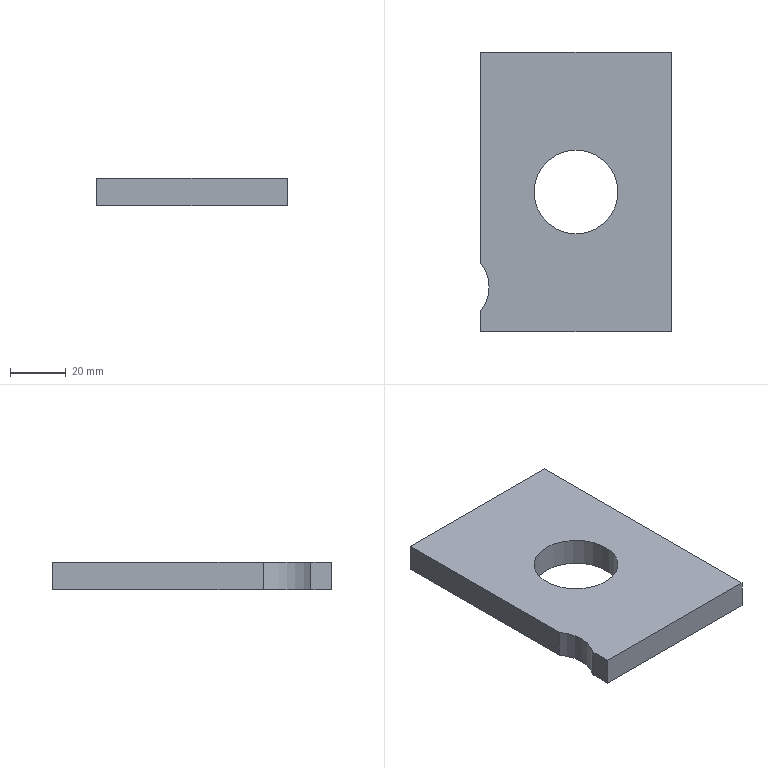Part | NX | features solid 2 | 1 solid | 9 faces | box 68 x 100 x 10 mm | volume 60595 mm3 | plane 7 | cylinder 2 | commonest cylinder face diameters 28 x1 30 x1
STEP:
#1=CARTESIAN_POINT('',(-550.,-16.475,-180.));
#2=VERTEX_POINT('',#1);
#3=CARTESIAN_POINT('',(-550.,-16.475,-190.));
#4=VERTEX_POINT('',#3);
#5=CARTESIAN_POINT('',(-550.,-16.475,320.));
#6=DIRECTION('',(0.,0.,-1.));
#7=VECTOR('',#6,1000.);
#8=LINE('',#5,#7);
#9=EDGE_CURVE('',#2,#4,#8,.T.);
#10=ORIENTED_EDGE('',*,*,#9,.F.);
#11=CARTESIAN_POINT('',(-550.,59.,-180.));
#12=VERTEX_POINT('',#11);
#13=CARTESIAN_POINT('',(-550.,-31.,-180.));
#14=DIRECTION('',(0.,-1.,0.));
#15=VECTOR('',#14,1000.);
#16=LINE('',#13,#15);
#17=EDGE_CURVE('',#12,#2,#16,.T.);
#18=ORIENTED_EDGE('',*,*,#17,.F.);
#19=CARTESIAN_POINT('',(-550.,59.,-190.));
#20=VERTEX_POINT('',#19);
#21=CARTESIAN_POINT('',(-550.,59.,-190.));
#22=DIRECTION('',(0.,0.,1.));
#23=VECTOR('',#22,1000.);
#24=LINE('',#21,#23);
#25=EDGE_CURVE('',#20,#12,#24,.T.);
#26=ORIENTED_EDGE('',*,*,#25,.F.);
#27=CARTESIAN_POINT('',(-550.,-31.,-190.));
#28=DIRECTION('',(0.,-1.,0.));
#29=VECTOR('',#28,1000.);
#30=LINE('',#27,#29);
#31=EDGE_CURVE('',#20,#4,#30,.T.);
#32=ORIENTED_EDGE('',*,*,#31,.T.);
#33=EDGE_LOOP('',(#10,#18,#26,#32));
#34=FACE_BOUND('',#33,.T.);
#35=CARTESIAN_POINT('',(-550.,49.,-190.));
#36=DIRECTION('',(-1.,0.,0.));
#37=DIRECTION('',(0.,-1.,0.));
#38=AXIS2_PLACEMENT_3D('',#35,#36,#37);
#39=PLANE('',#38);
#40=ADVANCED_FACE('',(#34),#39,.T.);
#41=CARTESIAN_POINT('',(-482.,59.,-180.));
#42=VERTEX_POINT('',#41);
#43=CARTESIAN_POINT('',(-482.,-41.,-180.));
#44=VERTEX_POINT('',#43);
#45=CARTESIAN_POINT('',(-482.,-31.,-180.));
#46=DIRECTION('',(0.,-1.,0.));
#47=VECTOR('',#46,1000.);
#48=LINE('',#45,#47);
#49=EDGE_CURVE('',#42,#44,#48,.T.);
#50=ORIENTED_EDGE('',*,*,#49,.T.);
#51=CARTESIAN_POINT('',(-482.,-41.,-190.));
#52=VERTEX_POINT('',#51);
#53=CARTESIAN_POINT('',(-482.,-41.,-190.));
#54=DIRECTION('',(0.,0.,1.));
#55=VECTOR('',#54,1000.);
#56=LINE('',#53,#55);
#57=EDGE_CURVE('',#52,#44,#56,.T.);
#58=ORIENTED_EDGE('',*,*,#57,.F.);
#59=CARTESIAN_POINT('',(-482.,59.,-190.));
#60=VERTEX_POINT('',#59);
#61=CARTESIAN_POINT('',(-482.,-31.,-190.));
#62=DIRECTION('',(0.,-1.,0.));
#63=VECTOR('',#62,1000.);
#64=LINE('',#61,#63);
#65=EDGE_CURVE('',#60,#52,#64,.T.);
#66=ORIENTED_EDGE('',*,*,#65,.F.);
#67=CARTESIAN_POINT('',(-482.,59.,-190.));
#68=DIRECTION('',(0.,0.,1.));
#69=VECTOR('',#68,1000.);
#70=LINE('',#67,#69);
#71=EDGE_CURVE('',#60,#42,#70,.T.);
#72=ORIENTED_EDGE('',*,*,#71,.T.);
#73=EDGE_LOOP('',(#50,#58,#66,#72));
#74=FACE_BOUND('',#73,.T.);
#75=CARTESIAN_POINT('',(-482.,49.,-190.));
#76=DIRECTION('',(-1.,0.,0.));
#77=DIRECTION('',(0.,0.,-1.));
#78=AXIS2_PLACEMENT_3D('',#75,#76,#77);
#79=PLANE('',#78);
#80=ADVANCED_FACE('',(#74),#79,.F.);
#81=CARTESIAN_POINT('',(-550.,-41.,-180.));
#82=VERTEX_POINT('',#81);
#83=CARTESIAN_POINT('',(-492.,-41.,-180.));
#84=DIRECTION('',(-1.,0.,0.));
#85=VECTOR('',#84,1000.);
#86=LINE('',#83,#85);
#87=EDGE_CURVE('',#44,#82,#86,.T.);
#88=ORIENTED_EDGE('',*,*,#87,.T.);
#89=CARTESIAN_POINT('',(-550.,-41.,-190.));
#90=VERTEX_POINT('',#89);
#91=CARTESIAN_POINT('',(-550.,-41.,-190.));
#92=DIRECTION('',(0.,0.,1.));
#93=VECTOR('',#92,1000.);
#94=LINE('',#91,#93);
#95=EDGE_CURVE('',#90,#82,#94,.T.);
#96=ORIENTED_EDGE('',*,*,#95,.F.);
#97=CARTESIAN_POINT('',(-492.,-41.,-190.));
#98=DIRECTION('',(-1.,0.,0.));
#99=VECTOR('',#98,1000.);
#100=LINE('',#97,#99);
#101=EDGE_CURVE('',#52,#90,#100,.T.);
#102=ORIENTED_EDGE('',*,*,#101,.F.);
#103=ORIENTED_EDGE('',*,*,#57,.T.);
#104=EDGE_LOOP('',(#88,#96,#102,#103));
#105=FACE_BOUND('',#104,.T.);
#106=CARTESIAN_POINT('',(-492.,-41.,-190.));
#107=DIRECTION('',(0.,1.,0.));
#108=DIRECTION('',(0.,0.,1.));
#109=AXIS2_PLACEMENT_3D('',#106,#107,#108);
#110=PLANE('',#109);
#111=ADVANCED_FACE('',(#105),#110,.F.);
#112=CARTESIAN_POINT('',(-550.,-33.525,-190.));
#113=VERTEX_POINT('',#112);
#114=CARTESIAN_POINT('',(-550.,-33.525,-180.));
#115=VERTEX_POINT('',#114);
#116=CARTESIAN_POINT('',(-550.,-33.525,320.));
#117=DIRECTION('',(0.,0.,-1.));
#118=VECTOR('',#117,1000.);
#119=LINE('',#116,#118);
#120=EDGE_CURVE('',#113,#115,#119,.F.);
#121=ORIENTED_EDGE('',*,*,#120,.F.);
#122=CARTESIAN_POINT('',(-550.,-31.,-190.));
#123=DIRECTION('',(0.,-1.,0.));
#124=VECTOR('',#123,1000.);
#125=LINE('',#122,#124);
#126=EDGE_CURVE('',#113,#90,#125,.T.);
#127=ORIENTED_EDGE('',*,*,#126,.T.);
#128=ORIENTED_EDGE('',*,*,#95,.T.);
#129=CARTESIAN_POINT('',(-550.,-31.,-180.));
#130=DIRECTION('',(0.,-1.,0.));
#131=VECTOR('',#130,1000.);
#132=LINE('',#129,#131);
#133=EDGE_CURVE('',#115,#82,#132,.T.);
#134=ORIENTED_EDGE('',*,*,#133,.F.);
#135=EDGE_LOOP('',(#121,#127,#128,#134));
#136=FACE_BOUND('',#135,.T.);
#137=CARTESIAN_POINT('',(-550.,49.,-190.));
#138=DIRECTION('',(-1.,0.,0.));
#139=DIRECTION('',(0.,-1.,0.));
#140=AXIS2_PLACEMENT_3D('',#137,#138,#139);
#141=PLANE('',#140);
#142=ADVANCED_FACE('',(#136),#141,.T.);
#143=CARTESIAN_POINT('',(-492.,59.,-180.));
#144=DIRECTION('',(-1.,0.,0.));
#145=VECTOR('',#144,1000.);
#146=LINE('',#143,#145);
#147=EDGE_CURVE('',#42,#12,#146,.T.);
#148=ORIENTED_EDGE('',*,*,#147,.F.);
#149=ORIENTED_EDGE('',*,*,#71,.F.);
#150=CARTESIAN_POINT('',(-492.,59.,-190.));
#151=DIRECTION('',(-1.,0.,0.));
#152=VECTOR('',#151,1000.);
#153=LINE('',#150,#152);
#154=EDGE_CURVE('',#60,#20,#153,.T.);
#155=ORIENTED_EDGE('',*,*,#154,.T.);
#156=ORIENTED_EDGE('',*,*,#25,.T.);
#157=EDGE_LOOP('',(#148,#149,#155,#156));
#158=FACE_BOUND('',#157,.T.);
#159=CARTESIAN_POINT('',(-492.,59.,-190.));
#160=DIRECTION('',(0.,1.,0.));
#161=DIRECTION('',(0.,0.,1.));
#162=AXIS2_PLACEMENT_3D('',#159,#160,#161);
#163=PLANE('',#162);
#164=ADVANCED_FACE('',(#158),#163,.T.);
#165=CARTESIAN_POINT('',(-516.,-6.,-190.));
#166=VERTEX_POINT('',#165);
#167=CARTESIAN_POINT('',(-516.,9.,-190.));
#168=DIRECTION('',(0.,0.,1.));
#169=DIRECTION('',(0.,-1.,0.));
#170=AXIS2_PLACEMENT_3D('',#167,#168,#169);
#171=CIRCLE('',#170,15.);
#172=EDGE_CURVE('',#166,#166,#171,.T.);
#173=ORIENTED_EDGE('',*,*,#172,.T.);
#174=EDGE_LOOP('',(#173));
#175=FACE_BOUND('',#174,.T.);
#176=ORIENTED_EDGE('',*,*,#126,.F.);
#177=CARTESIAN_POINT('',(-561.105,-25.,-190.));
#178=DIRECTION('',(0.,0.,1.));
#179=DIRECTION('',(1.,0.,0.));
#180=AXIS2_PLACEMENT_3D('',#177,#178,#179);
#181=CIRCLE('',#180,14.);
#182=EDGE_CURVE('',#113,#4,#181,.T.);
#183=ORIENTED_EDGE('',*,*,#182,.T.);
#184=ORIENTED_EDGE('',*,*,#31,.F.);
#185=ORIENTED_EDGE('',*,*,#154,.F.);
#186=ORIENTED_EDGE('',*,*,#65,.T.);
#187=ORIENTED_EDGE('',*,*,#101,.T.);
#188=EDGE_LOOP('',(#176,#183,#184,#185,#186,#187));
#189=FACE_BOUND('',#188,.T.);
#190=CARTESIAN_POINT('',(-492.,-31.,-190.));
#191=DIRECTION('',(0.,0.,1.));
#192=DIRECTION('',(0.,-1.,0.));
#193=AXIS2_PLACEMENT_3D('',#190,#191,#192);
#194=PLANE('',#193);
#195=ADVANCED_FACE('',(#175,#189),#194,.F.);
#196=CARTESIAN_POINT('',(-561.105,-25.,-180.));
#197=DIRECTION('',(0.,0.,1.));
#198=DIRECTION('',(1.,0.,0.));
#199=AXIS2_PLACEMENT_3D('',#196,#197,#198);
#200=CIRCLE('',#199,14.);
#201=EDGE_CURVE('',#115,#2,#200,.T.);
#202=ORIENTED_EDGE('',*,*,#201,.F.);
#203=ORIENTED_EDGE('',*,*,#133,.T.);
#204=ORIENTED_EDGE('',*,*,#87,.F.);
#205=ORIENTED_EDGE('',*,*,#49,.F.);
#206=ORIENTED_EDGE('',*,*,#147,.T.);
#207=ORIENTED_EDGE('',*,*,#17,.T.);
#208=EDGE_LOOP('',(#202,#203,#204,#205,#206,#207));
#209=FACE_BOUND('',#208,.T.);
#210=CARTESIAN_POINT('',(-516.,-6.,-180.));
#211=VERTEX_POINT('',#210);
#212=CARTESIAN_POINT('',(-516.,9.,-180.));
#213=DIRECTION('',(0.,0.,1.));
#214=DIRECTION('',(0.,-1.,0.));
#215=AXIS2_PLACEMENT_3D('',#212,#213,#214);
#216=CIRCLE('',#215,15.);
#217=EDGE_CURVE('',#211,#211,#216,.T.);
#218=ORIENTED_EDGE('',*,*,#217,.F.);
#219=EDGE_LOOP('',(#218));
#220=FACE_BOUND('',#219,.T.);
#221=CARTESIAN_POINT('',(-492.,-31.,-180.));
#222=DIRECTION('',(0.,0.,1.));
#223=DIRECTION('',(0.,-1.,0.));
#224=AXIS2_PLACEMENT_3D('',#221,#222,#223);
#225=PLANE('',#224);
#226=ADVANCED_FACE('',(#209,#220),#225,.T.);
#227=ORIENTED_EDGE('',*,*,#217,.T.);
#228=EDGE_LOOP('',(#227));
#229=FACE_BOUND('',#228,.T.);
#230=ORIENTED_EDGE('',*,*,#172,.F.);
#231=EDGE_LOOP('',(#230));
#232=FACE_BOUND('',#231,.T.);
#233=CARTESIAN_POINT('',(-516.,9.,-186.));
#234=DIRECTION('',(0.,0.,1.));
#235=DIRECTION('',(0.,-1.,0.));
#236=AXIS2_PLACEMENT_3D('',#233,#234,#235);
#237=CYLINDRICAL_SURFACE('',#236,15.);
#238=ADVANCED_FACE('',(#229,#232),#237,.F.);
#239=ORIENTED_EDGE('',*,*,#120,.T.);
#240=ORIENTED_EDGE('',*,*,#201,.T.);
#241=ORIENTED_EDGE('',*,*,#9,.T.);
#242=ORIENTED_EDGE('',*,*,#182,.F.);
#243=EDGE_LOOP('',(#239,#240,#241,#242));
#244=FACE_BOUND('',#243,.T.);
#245=CARTESIAN_POINT('',(-561.105,-25.,320.));
#246=DIRECTION('',(0.,0.,-1.));
#247=DIRECTION('',(-1.,0.,0.));
#248=AXIS2_PLACEMENT_3D('',#245,#246,#247);
#249=CYLINDRICAL_SURFACE('',#248,14.);
#250=ADVANCED_FACE('',(#244),#249,.F.);
#251=CLOSED_SHELL('',(#40,#80,#111,#142,#164,#195,#226,#238,#250));
#252=MANIFOLD_SOLID_BREP('',#251);
#253=(LENGTH_UNIT()NAMED_UNIT(*)SI_UNIT(.MILLI.,.METRE.));
#254=UNCERTAINTY_MEASURE_WITH_UNIT(LENGTH_MEASURE(0.00001),#253,'','');
#255=(NAMED_UNIT(*)PLANE_ANGLE_UNIT()SI_UNIT($,.RADIAN.));
#256=(NAMED_UNIT(*)SI_UNIT($,.STERADIAN.)SOLID_ANGLE_UNIT());
#257=(GEOMETRIC_REPRESENTATION_CONTEXT(3)GLOBAL_UNCERTAINTY_ASSIGNED_CONTEXT((#254))GLOBAL_UNIT_ASSIGNED_CONTEXT((#253,#255,#256))REPRESENTATION_CONTEXT('',''));
#258=ADVANCED_BREP_SHAPE_REPRESENTATION('',(#252),#257);